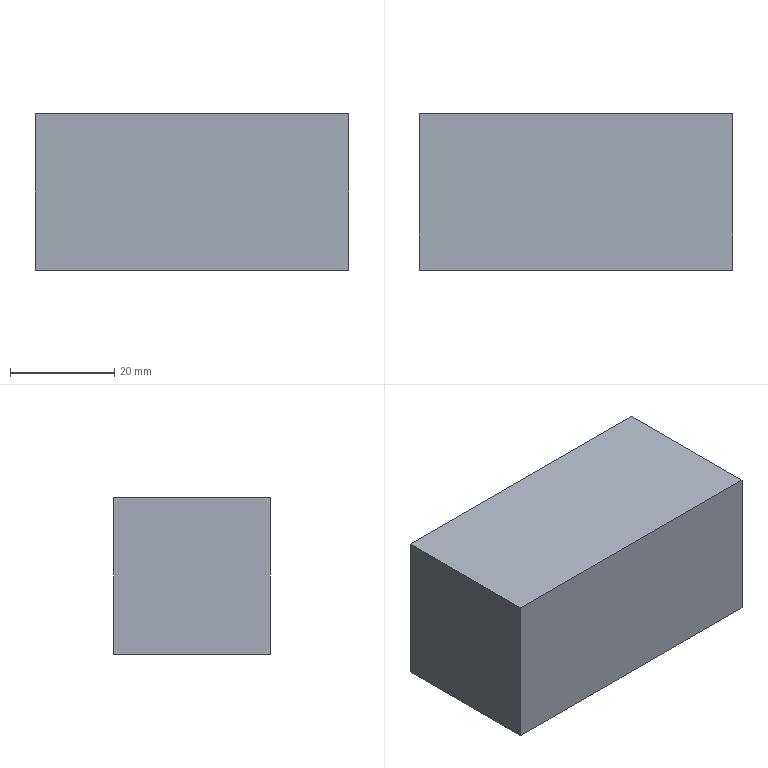Part | SolidWorks | features Extrusion 1 | 1 solid | 6 faces | box 60 x 30 x 30 mm | volume 54000 mm3 | plane 6
STEP:
#1=CARTESIAN_POINT('',(0.,30.,0.));
#2=VERTEX_POINT('',#1);
#3=CARTESIAN_POINT('',(0.,0.,0.));
#4=VERTEX_POINT('',#3);
#5=CARTESIAN_POINT('',(0.,0.,0.));
#6=DIRECTION('',(0.,-1.,0.));
#7=VECTOR('',#6,1000.);
#8=LINE('',#5,#7);
#9=EDGE_CURVE('',#2,#4,#8,.T.);
#10=ORIENTED_EDGE('',*,*,#9,.T.);
#11=CARTESIAN_POINT('',(0.,0.,30.));
#12=VERTEX_POINT('',#11);
#13=CARTESIAN_POINT('',(0.,0.,30.));
#14=DIRECTION('',(0.,0.,-1.));
#15=VECTOR('',#14,1000.);
#16=LINE('',#13,#15);
#17=EDGE_CURVE('',#12,#4,#16,.T.);
#18=ORIENTED_EDGE('',*,*,#17,.F.);
#19=CARTESIAN_POINT('',(0.,30.,30.));
#20=VERTEX_POINT('',#19);
#21=CARTESIAN_POINT('',(0.,0.,30.));
#22=DIRECTION('',(0.,-1.,0.));
#23=VECTOR('',#22,1000.);
#24=LINE('',#21,#23);
#25=EDGE_CURVE('',#20,#12,#24,.T.);
#26=ORIENTED_EDGE('',*,*,#25,.F.);
#27=CARTESIAN_POINT('',(0.,30.,30.));
#28=DIRECTION('',(0.,0.,-1.));
#29=VECTOR('',#28,1000.);
#30=LINE('',#27,#29);
#31=EDGE_CURVE('',#20,#2,#30,.T.);
#32=ORIENTED_EDGE('',*,*,#31,.T.);
#33=EDGE_LOOP('',(#10,#18,#26,#32));
#34=FACE_OUTER_BOUND('',#33,.T.);
#35=CARTESIAN_POINT('',(0.,0.,30.));
#36=DIRECTION('',(1.,0.,0.));
#37=DIRECTION('',(0.,0.,-1.));
#38=AXIS2_PLACEMENT_3D('',#35,#36,#37);
#39=PLANE('',#38);
#40=ADVANCED_FACE('',(#34),#39,.F.);
#41=CARTESIAN_POINT('',(60.,0.,0.));
#42=VERTEX_POINT('',#41);
#43=CARTESIAN_POINT('',(0.,0.,0.));
#44=DIRECTION('',(1.,0.,0.));
#45=VECTOR('',#44,1000.);
#46=LINE('',#43,#45);
#47=EDGE_CURVE('',#4,#42,#46,.T.);
#48=ORIENTED_EDGE('',*,*,#47,.T.);
#49=CARTESIAN_POINT('',(60.,0.,30.));
#50=VERTEX_POINT('',#49);
#51=CARTESIAN_POINT('',(60.,0.,30.));
#52=DIRECTION('',(0.,0.,-1.));
#53=VECTOR('',#52,1000.);
#54=LINE('',#51,#53);
#55=EDGE_CURVE('',#50,#42,#54,.T.);
#56=ORIENTED_EDGE('',*,*,#55,.F.);
#57=CARTESIAN_POINT('',(0.,0.,30.));
#58=DIRECTION('',(1.,0.,0.));
#59=VECTOR('',#58,1000.);
#60=LINE('',#57,#59);
#61=EDGE_CURVE('',#12,#50,#60,.T.);
#62=ORIENTED_EDGE('',*,*,#61,.F.);
#63=ORIENTED_EDGE('',*,*,#17,.T.);
#64=EDGE_LOOP('',(#48,#56,#62,#63));
#65=FACE_OUTER_BOUND('',#64,.T.);
#66=CARTESIAN_POINT('',(0.,0.,30.));
#67=DIRECTION('',(0.,1.,0.));
#68=DIRECTION('',(0.,0.,1.));
#69=AXIS2_PLACEMENT_3D('',#66,#67,#68);
#70=PLANE('',#69);
#71=ADVANCED_FACE('',(#65),#70,.F.);
#72=CARTESIAN_POINT('',(60.,30.,0.));
#73=VERTEX_POINT('',#72);
#74=CARTESIAN_POINT('',(60.,0.,0.));
#75=DIRECTION('',(0.,1.,0.));
#76=VECTOR('',#75,1000.);
#77=LINE('',#74,#76);
#78=EDGE_CURVE('',#42,#73,#77,.T.);
#79=ORIENTED_EDGE('',*,*,#78,.T.);
#80=CARTESIAN_POINT('',(60.,30.,30.));
#81=VERTEX_POINT('',#80);
#82=CARTESIAN_POINT('',(60.,30.,30.));
#83=DIRECTION('',(0.,0.,-1.));
#84=VECTOR('',#83,1000.);
#85=LINE('',#82,#84);
#86=EDGE_CURVE('',#81,#73,#85,.T.);
#87=ORIENTED_EDGE('',*,*,#86,.F.);
#88=CARTESIAN_POINT('',(60.,0.,30.));
#89=DIRECTION('',(0.,1.,0.));
#90=VECTOR('',#89,1000.);
#91=LINE('',#88,#90);
#92=EDGE_CURVE('',#50,#81,#91,.T.);
#93=ORIENTED_EDGE('',*,*,#92,.F.);
#94=ORIENTED_EDGE('',*,*,#55,.T.);
#95=EDGE_LOOP('',(#79,#87,#93,#94));
#96=FACE_OUTER_BOUND('',#95,.T.);
#97=CARTESIAN_POINT('',(60.,0.,30.));
#98=DIRECTION('',(-1.,0.,0.));
#99=DIRECTION('',(0.,0.,1.));
#100=AXIS2_PLACEMENT_3D('',#97,#98,#99);
#101=PLANE('',#100);
#102=ADVANCED_FACE('',(#96),#101,.F.);
#103=CARTESIAN_POINT('',(0.,30.,0.));
#104=DIRECTION('',(-1.,0.,0.));
#105=VECTOR('',#104,1000.);
#106=LINE('',#103,#105);
#107=EDGE_CURVE('',#73,#2,#106,.T.);
#108=ORIENTED_EDGE('',*,*,#107,.T.);
#109=ORIENTED_EDGE('',*,*,#31,.F.);
#110=CARTESIAN_POINT('',(0.,30.,30.));
#111=DIRECTION('',(-1.,0.,0.));
#112=VECTOR('',#111,1000.);
#113=LINE('',#110,#112);
#114=EDGE_CURVE('',#81,#20,#113,.T.);
#115=ORIENTED_EDGE('',*,*,#114,.F.);
#116=ORIENTED_EDGE('',*,*,#86,.T.);
#117=EDGE_LOOP('',(#108,#109,#115,#116));
#118=FACE_OUTER_BOUND('',#117,.T.);
#119=CARTESIAN_POINT('',(0.,30.,30.));
#120=DIRECTION('',(0.,-1.,0.));
#121=DIRECTION('',(0.,0.,-1.));
#122=AXIS2_PLACEMENT_3D('',#119,#120,#121);
#123=PLANE('',#122);
#124=ADVANCED_FACE('',(#118),#123,.F.);
#125=ORIENTED_EDGE('',*,*,#25,.T.);
#126=ORIENTED_EDGE('',*,*,#61,.T.);
#127=ORIENTED_EDGE('',*,*,#92,.T.);
#128=ORIENTED_EDGE('',*,*,#114,.T.);
#129=EDGE_LOOP('',(#125,#126,#127,#128));
#130=FACE_OUTER_BOUND('',#129,.T.);
#131=CARTESIAN_POINT('',(0.,0.,30.));
#132=DIRECTION('',(0.,0.,-1.));
#133=DIRECTION('',(-1.,0.,0.));
#134=AXIS2_PLACEMENT_3D('',#131,#132,#133);
#135=PLANE('',#134);
#136=ADVANCED_FACE('',(#130),#135,.F.);
#137=ORIENTED_EDGE('',*,*,#9,.F.);
#138=ORIENTED_EDGE('',*,*,#107,.F.);
#139=ORIENTED_EDGE('',*,*,#78,.F.);
#140=ORIENTED_EDGE('',*,*,#47,.F.);
#141=EDGE_LOOP('',(#137,#138,#139,#140));
#142=FACE_OUTER_BOUND('',#141,.T.);
#143=CARTESIAN_POINT('',(0.,0.,0.));
#144=DIRECTION('',(0.,0.,-1.));
#145=DIRECTION('',(-1.,0.,0.));
#146=AXIS2_PLACEMENT_3D('',#143,#144,#145);
#147=PLANE('',#146);
#148=ADVANCED_FACE('',(#142),#147,.T.);
#149=CLOSED_SHELL('',(#40,#71,#102,#124,#136,#148));
#150=MANIFOLD_SOLID_BREP('',#149);
#151=CARTESIAN_POINT('',(0.,0.,0.));
#152=DIRECTION('',(0.,0.,1.));
#153=DIRECTION('',(1.,0.,0.));
#154=AXIS2_PLACEMENT_3D('',#151,#152,#153);
#155=(LENGTH_UNIT()NAMED_UNIT(*)SI_UNIT(.MILLI.,.METRE.));
#156=UNCERTAINTY_MEASURE_WITH_UNIT(LENGTH_MEASURE(0.00001),#155,'','');
#157=(NAMED_UNIT(*)PLANE_ANGLE_UNIT()SI_UNIT($,.RADIAN.));
#158=(NAMED_UNIT(*)SI_UNIT($,.STERADIAN.)SOLID_ANGLE_UNIT());
#159=(GEOMETRIC_REPRESENTATION_CONTEXT(3)GLOBAL_UNCERTAINTY_ASSIGNED_CONTEXT((#156))GLOBAL_UNIT_ASSIGNED_CONTEXT((#155,#157,#158))REPRESENTATION_CONTEXT('',''));
#160=ADVANCED_BREP_SHAPE_REPRESENTATION('',(#150,#154),#159);